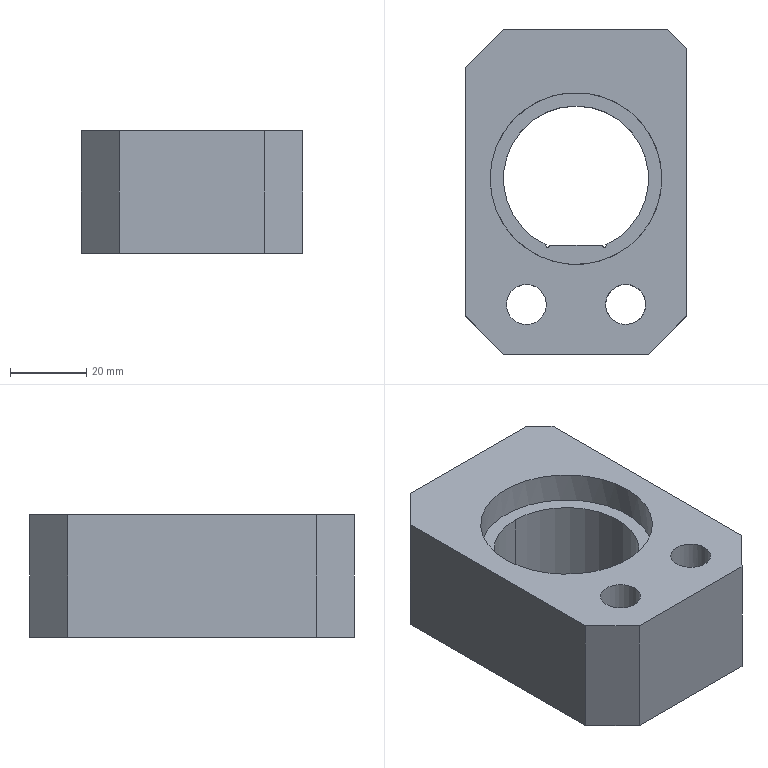Part | STEP file | lll_id3674_x_t | 1 solid | 23 faces | box 58 x 85 x 32 mm | volume 102639 mm3 | plane 14 | cylinder 9 | commonest cylinder face diameters 1 x2 10.5 x2 17 x2 38 x2 45 x1
STEP:
#1=CARTESIAN_POINT('',(3397.,-57.,84.5));
#2=VERTEX_POINT('',#1);
#3=CARTESIAN_POINT('',(3419.5,-57.,84.5));
#4=DIRECTION('',(0.,0.,-1.));
#5=DIRECTION('',(-1.,0.,0.));
#6=AXIS2_PLACEMENT_3D('',#3,#4,#5);
#7=CIRCLE('',#6,22.5);
#8=EDGE_CURVE('',#2,#2,#7,.T.);
#9=ORIENTED_EDGE('',*,*,#8,.F.);
#10=EDGE_LOOP('',(#9));
#11=FACE_BOUND('',#10,.T.);
#12=CARTESIAN_POINT('',(3426.399,-74.5,84.5));
#13=VERTEX_POINT('',#12);
#14=CARTESIAN_POINT('',(3427.357,-74.299,84.5));
#15=VERTEX_POINT('',#14);
#16=CARTESIAN_POINT('',(3426.899,-74.5,84.5));
#17=DIRECTION('',(0.,0.,1.));
#18=DIRECTION('',(-1.,0.,0.));
#19=AXIS2_PLACEMENT_3D('',#16,#17,#18);
#20=CIRCLE('',#19,0.5);
#21=EDGE_CURVE('',#13,#15,#20,.T.);
#22=ORIENTED_EDGE('',*,*,#21,.F.);
#23=CARTESIAN_POINT('',(3412.601,-74.5,84.5));
#24=VERTEX_POINT('',#23);
#25=CARTESIAN_POINT('',(3399.25,-74.5,84.5));
#26=DIRECTION('',(-1.,0.,0.));
#27=VECTOR('',#26,1.);
#28=LINE('',#25,#27);
#29=EDGE_CURVE('',#13,#24,#28,.T.);
#30=ORIENTED_EDGE('',*,*,#29,.T.);
#31=CARTESIAN_POINT('',(3411.643,-74.299,84.5));
#32=VERTEX_POINT('',#31);
#33=CARTESIAN_POINT('',(3412.101,-74.5,84.5));
#34=DIRECTION('',(0.,0.,-1.));
#35=DIRECTION('',(1.,0.,0.));
#36=AXIS2_PLACEMENT_3D('',#33,#34,#35);
#37=CIRCLE('',#36,0.5);
#38=EDGE_CURVE('',#24,#32,#37,.T.);
#39=ORIENTED_EDGE('',*,*,#38,.T.);
#40=CARTESIAN_POINT('',(3419.5,-38.,84.5));
#41=VERTEX_POINT('',#40);
#42=CARTESIAN_POINT('',(3419.5,-57.,84.5));
#43=DIRECTION('',(0.,0.,1.));
#44=DIRECTION('',(0.,1.,0.));
#45=AXIS2_PLACEMENT_3D('',#42,#43,#44);
#46=CIRCLE('',#45,19.);
#47=EDGE_CURVE('',#41,#32,#46,.T.);
#48=ORIENTED_EDGE('',*,*,#47,.F.);
#49=CARTESIAN_POINT('',(3419.5,-57.,84.5));
#50=DIRECTION('',(0.,0.,1.));
#51=DIRECTION('',(0.,1.,0.));
#52=AXIS2_PLACEMENT_3D('',#49,#50,#51);
#53=CIRCLE('',#52,19.);
#54=EDGE_CURVE('',#15,#41,#53,.T.);
#55=ORIENTED_EDGE('',*,*,#54,.F.);
#56=EDGE_LOOP('',(#22,#30,#39,#48,#55));
#57=FACE_BOUND('',#56,.T.);
#58=CARTESIAN_POINT('',(3399.25,-57.,84.5));
#59=DIRECTION('',(0.,0.,-1.));
#60=DIRECTION('',(-1.,0.,0.));
#61=AXIS2_PLACEMENT_3D('',#58,#59,#60);
#62=PLANE('',#61);
#63=ADVANCED_FACE('',(#11,#57),#62,.F.);
#64=CARTESIAN_POINT('',(3406.5,-84.75,77.5));
#65=VERTEX_POINT('',#64);
#66=CARTESIAN_POINT('',(3406.5,-90.,77.5));
#67=DIRECTION('',(0.,0.,1.));
#68=DIRECTION('',(0.,1.,0.));
#69=AXIS2_PLACEMENT_3D('',#66,#67,#68);
#70=CIRCLE('',#69,5.25);
#71=EDGE_CURVE('',#65,#65,#70,.T.);
#72=ORIENTED_EDGE('',*,*,#71,.T.);
#73=EDGE_LOOP('',(#72));
#74=FACE_BOUND('',#73,.T.);
#75=CARTESIAN_POINT('',(3406.5,-81.5,77.5));
#76=VERTEX_POINT('',#75);
#77=CARTESIAN_POINT('',(3406.5,-90.,77.5));
#78=DIRECTION('',(0.,0.,1.));
#79=DIRECTION('',(0.,1.,0.));
#80=AXIS2_PLACEMENT_3D('',#77,#78,#79);
#81=CIRCLE('',#80,8.5);
#82=EDGE_CURVE('',#76,#76,#81,.T.);
#83=ORIENTED_EDGE('',*,*,#82,.F.);
#84=EDGE_LOOP('',(#83));
#85=FACE_BOUND('',#84,.T.);
#86=CARTESIAN_POINT('',(3406.5,-90.,77.5));
#87=DIRECTION('',(0.,0.,1.));
#88=DIRECTION('',(1.,0.,0.));
#89=AXIS2_PLACEMENT_3D('',#86,#87,#88);
#90=PLANE('',#89);
#91=ADVANCED_FACE('',(#74,#85),#90,.F.);
#92=ORIENTED_EDGE('',*,*,#82,.T.);
#93=EDGE_LOOP('',(#92));
#94=FACE_BOUND('',#93,.T.);
#95=CARTESIAN_POINT('',(3406.5,-81.5,60.5));
#96=VERTEX_POINT('',#95);
#97=CARTESIAN_POINT('',(3406.5,-90.,60.5));
#98=DIRECTION('',(0.,0.,-1.));
#99=DIRECTION('',(0.,1.,0.));
#100=AXIS2_PLACEMENT_3D('',#97,#98,#99);
#101=CIRCLE('',#100,8.5);
#102=EDGE_CURVE('',#96,#96,#101,.T.);
#103=ORIENTED_EDGE('',*,*,#102,.T.);
#104=EDGE_LOOP('',(#103));
#105=FACE_BOUND('',#104,.T.);
#106=CARTESIAN_POINT('',(3406.5,-90.,60.5));
#107=DIRECTION('',(0.,0.,1.));
#108=DIRECTION('',(1.,0.,0.));
#109=AXIS2_PLACEMENT_3D('',#106,#107,#108);
#110=CYLINDRICAL_SURFACE('',#109,8.5);
#111=ADVANCED_FACE('',(#94,#105),#110,.F.);
#112=CARTESIAN_POINT('',(3400.5,-103.,60.5));
#113=VERTEX_POINT('',#112);
#114=CARTESIAN_POINT('',(3390.5,-93.,60.5));
#115=VERTEX_POINT('',#114);
#116=CARTESIAN_POINT('',(3430.983,-133.483,60.5));
#117=DIRECTION('',(-0.7071,0.7071,0.));
#118=VECTOR('',#117,1.);
#119=LINE('',#116,#118);
#120=EDGE_CURVE('',#113,#115,#119,.T.);
#121=ORIENTED_EDGE('',*,*,#120,.F.);
#122=CARTESIAN_POINT('',(3400.5,-103.,92.5));
#123=VERTEX_POINT('',#122);
#124=CARTESIAN_POINT('',(3400.5,-103.,-8.5));
#125=DIRECTION('',(0.,0.,-1.));
#126=VECTOR('',#125,1.);
#127=LINE('',#124,#126);
#128=EDGE_CURVE('',#123,#113,#127,.T.);
#129=ORIENTED_EDGE('',*,*,#128,.F.);
#130=CARTESIAN_POINT('',(3390.5,-93.,92.5));
#131=VERTEX_POINT('',#130);
#132=CARTESIAN_POINT('',(3435.933,-138.433,92.5));
#133=DIRECTION('',(0.7071,-0.7071,0.));
#134=VECTOR('',#133,1.);
#135=LINE('',#132,#134);
#136=EDGE_CURVE('',#131,#123,#135,.T.);
#137=ORIENTED_EDGE('',*,*,#136,.F.);
#138=CARTESIAN_POINT('',(3390.5,-93.,-8.5));
#139=DIRECTION('',(0.,0.,1.));
#140=VECTOR('',#139,1.);
#141=LINE('',#138,#140);
#142=EDGE_CURVE('',#115,#131,#141,.T.);
#143=ORIENTED_EDGE('',*,*,#142,.F.);
#144=EDGE_LOOP('',(#121,#129,#137,#143));
#145=FACE_OUTER_BOUND('',#144,.T.);
#146=CARTESIAN_POINT('',(3390.5,-93.,-8.5));
#147=DIRECTION('',(0.7071,0.7071,0.));
#148=DIRECTION('',(0.,0.,1.));
#149=AXIS2_PLACEMENT_3D('',#146,#147,#148);
#150=PLANE('',#149);
#151=ADVANCED_FACE('',(#145),#150,.F.);
#152=CARTESIAN_POINT('',(3390.5,-28.,60.5));
#153=VERTEX_POINT('',#152);
#154=CARTESIAN_POINT('',(3390.5,-83.276,60.5));
#155=DIRECTION('',(0.,1.,0.));
#156=VECTOR('',#155,1.);
#157=LINE('',#154,#156);
#158=EDGE_CURVE('',#115,#153,#157,.T.);
#159=ORIENTED_EDGE('',*,*,#158,.F.);
#160=ORIENTED_EDGE('',*,*,#142,.T.);
#161=CARTESIAN_POINT('',(3390.5,-28.,92.5));
#162=VERTEX_POINT('',#161);
#163=CARTESIAN_POINT('',(3390.5,-88.225,92.5));
#164=DIRECTION('',(0.,-1.,0.));
#165=VECTOR('',#164,1.);
#166=LINE('',#163,#165);
#167=EDGE_CURVE('',#162,#131,#166,.T.);
#168=ORIENTED_EDGE('',*,*,#167,.F.);
#169=CARTESIAN_POINT('',(3390.5,-28.,-8.5));
#170=DIRECTION('',(0.,0.,-1.));
#171=VECTOR('',#170,1.);
#172=LINE('',#169,#171);
#173=EDGE_CURVE('',#162,#153,#172,.T.);
#174=ORIENTED_EDGE('',*,*,#173,.T.);
#175=EDGE_LOOP('',(#159,#160,#168,#174));
#176=FACE_OUTER_BOUND('',#175,.T.);
#177=CARTESIAN_POINT('',(3390.5,-52.05,-8.5));
#178=DIRECTION('',(-1.,0.,0.));
#179=DIRECTION('',(0.,0.,1.));
#180=AXIS2_PLACEMENT_3D('',#177,#178,#179);
#181=PLANE('',#180);
#182=ADVANCED_FACE('',(#176),#181,.T.);
#183=CARTESIAN_POINT('',(3400.5,-18.,92.5));
#184=VERTEX_POINT('',#183);
#185=CARTESIAN_POINT('',(3414.207,-4.293,92.5));
#186=DIRECTION('',(-0.7071,-0.7071,0.));
#187=VECTOR('',#186,1.);
#188=LINE('',#185,#187);
#189=EDGE_CURVE('',#184,#162,#188,.T.);
#190=ORIENTED_EDGE('',*,*,#189,.F.);
#191=CARTESIAN_POINT('',(3400.5,-18.,60.5));
#192=VERTEX_POINT('',#191);
#193=CARTESIAN_POINT('',(3400.5,-18.,-8.5));
#194=DIRECTION('',(0.,0.,1.));
#195=VECTOR('',#194,1.);
#196=LINE('',#193,#195);
#197=EDGE_CURVE('',#192,#184,#196,.T.);
#198=ORIENTED_EDGE('',*,*,#197,.F.);
#199=CARTESIAN_POINT('',(3414.207,-4.293,60.5));
#200=DIRECTION('',(0.7071,0.7071,0.));
#201=VECTOR('',#200,1.);
#202=LINE('',#199,#201);
#203=EDGE_CURVE('',#153,#192,#202,.T.);
#204=ORIENTED_EDGE('',*,*,#203,.F.);
#205=ORIENTED_EDGE('',*,*,#173,.F.);
#206=EDGE_LOOP('',(#190,#198,#204,#205));
#207=FACE_OUTER_BOUND('',#206,.T.);
#208=CARTESIAN_POINT('',(3390.5,-28.,-8.5));
#209=DIRECTION('',(0.7071,-0.7071,0.));
#210=DIRECTION('',(0.,0.,-1.));
#211=AXIS2_PLACEMENT_3D('',#208,#209,#210);
#212=PLANE('',#211);
#213=ADVANCED_FACE('',(#207),#212,.F.);
#214=CARTESIAN_POINT('',(3443.5,-18.,92.5));
#215=VERTEX_POINT('',#214);
#216=CARTESIAN_POINT('',(3487.64,-18.,92.5));
#217=DIRECTION('',(-1.,0.,0.));
#218=VECTOR('',#217,1.);
#219=LINE('',#216,#218);
#220=EDGE_CURVE('',#215,#184,#219,.T.);
#221=ORIENTED_EDGE('',*,*,#220,.F.);
#222=CARTESIAN_POINT('',(3443.5,-18.,60.5));
#223=VERTEX_POINT('',#222);
#224=CARTESIAN_POINT('',(3443.5,-18.,-8.5));
#225=DIRECTION('',(0.,0.,-1.));
#226=VECTOR('',#225,1.);
#227=LINE('',#224,#226);
#228=EDGE_CURVE('',#215,#223,#227,.T.);
#229=ORIENTED_EDGE('',*,*,#228,.T.);
#230=CARTESIAN_POINT('',(3482.69,-18.,60.5));
#231=DIRECTION('',(1.,0.,0.));
#232=VECTOR('',#231,1.);
#233=LINE('',#230,#232);
#234=EDGE_CURVE('',#192,#223,#233,.T.);
#235=ORIENTED_EDGE('',*,*,#234,.F.);
#236=ORIENTED_EDGE('',*,*,#197,.T.);
#237=EDGE_LOOP('',(#221,#229,#235,#236));
#238=FACE_OUTER_BOUND('',#237,.T.);
#239=CARTESIAN_POINT('',(3419.5,-18.,-8.5));
#240=DIRECTION('',(0.,1.,0.));
#241=DIRECTION('',(0.,0.,-1.));
#242=AXIS2_PLACEMENT_3D('',#239,#240,#241);
#243=PLANE('',#242);
#244=ADVANCED_FACE('',(#238),#243,.T.);
#245=CARTESIAN_POINT('',(3448.5,-23.,92.5));
#246=VERTEX_POINT('',#245);
#247=CARTESIAN_POINT('',(3495.433,-69.933,92.5));
#248=DIRECTION('',(-0.7071,0.7071,0.));
#249=VECTOR('',#248,1.);
#250=LINE('',#247,#249);
#251=EDGE_CURVE('',#246,#215,#250,.T.);
#252=ORIENTED_EDGE('',*,*,#251,.F.);
#253=CARTESIAN_POINT('',(3448.5,-23.,60.5));
#254=VERTEX_POINT('',#253);
#255=CARTESIAN_POINT('',(3448.5,-23.,-8.5));
#256=DIRECTION('',(0.,0.,1.));
#257=VECTOR('',#256,1.);
#258=LINE('',#255,#257);
#259=EDGE_CURVE('',#254,#246,#258,.T.);
#260=ORIENTED_EDGE('',*,*,#259,.F.);
#261=CARTESIAN_POINT('',(3490.483,-64.983,60.5));
#262=DIRECTION('',(0.7071,-0.7071,0.));
#263=VECTOR('',#262,1.);
#264=LINE('',#261,#263);
#265=EDGE_CURVE('',#223,#254,#264,.T.);
#266=ORIENTED_EDGE('',*,*,#265,.F.);
#267=ORIENTED_EDGE('',*,*,#228,.F.);
#268=EDGE_LOOP('',(#252,#260,#266,#267));
#269=FACE_OUTER_BOUND('',#268,.T.);
#270=CARTESIAN_POINT('',(3443.5,-18.,-8.5));
#271=DIRECTION('',(-0.7071,-0.7071,0.));
#272=DIRECTION('',(0.,0.,-1.));
#273=AXIS2_PLACEMENT_3D('',#270,#271,#272);
#274=PLANE('',#273);
#275=ADVANCED_FACE('',(#269),#274,.F.);
#276=CARTESIAN_POINT('',(3448.5,-93.,92.5));
#277=VERTEX_POINT('',#276);
#278=CARTESIAN_POINT('',(3448.5,-88.225,92.5));
#279=DIRECTION('',(0.,1.,0.));
#280=VECTOR('',#279,1.);
#281=LINE('',#278,#280);
#282=EDGE_CURVE('',#277,#246,#281,.T.);
#283=ORIENTED_EDGE('',*,*,#282,.F.);
#284=CARTESIAN_POINT('',(3448.5,-93.,60.5));
#285=VERTEX_POINT('',#284);
#286=CARTESIAN_POINT('',(3448.5,-93.,-8.5));
#287=DIRECTION('',(0.,0.,-1.));
#288=VECTOR('',#287,1.);
#289=LINE('',#286,#288);
#290=EDGE_CURVE('',#277,#285,#289,.T.);
#291=ORIENTED_EDGE('',*,*,#290,.T.);
#292=CARTESIAN_POINT('',(3448.5,-83.276,60.5));
#293=DIRECTION('',(0.,-1.,0.));
#294=VECTOR('',#293,1.);
#295=LINE('',#292,#294);
#296=EDGE_CURVE('',#254,#285,#295,.T.);
#297=ORIENTED_EDGE('',*,*,#296,.F.);
#298=ORIENTED_EDGE('',*,*,#259,.T.);
#299=EDGE_LOOP('',(#283,#291,#297,#298));
#300=FACE_OUTER_BOUND('',#299,.T.);
#301=CARTESIAN_POINT('',(3448.5,-57.,-8.5));
#302=DIRECTION('',(1.,0.,0.));
#303=DIRECTION('',(0.,0.,-1.));
#304=AXIS2_PLACEMENT_3D('',#301,#302,#303);
#305=PLANE('',#304);
#306=ADVANCED_FACE('',(#300),#305,.T.);
#307=CARTESIAN_POINT('',(3438.5,-103.,92.5));
#308=VERTEX_POINT('',#307);
#309=CARTESIAN_POINT('',(3470.707,-70.793,92.5));
#310=DIRECTION('',(0.7071,0.7071,0.));
#311=VECTOR('',#310,1.);
#312=LINE('',#309,#311);
#313=EDGE_CURVE('',#308,#277,#312,.T.);
#314=ORIENTED_EDGE('',*,*,#313,.F.);
#315=CARTESIAN_POINT('',(3438.5,-103.,60.5));
#316=VERTEX_POINT('',#315);
#317=CARTESIAN_POINT('',(3438.5,-103.,-8.5));
#318=DIRECTION('',(0.,0.,1.));
#319=VECTOR('',#318,1.);
#320=LINE('',#317,#319);
#321=EDGE_CURVE('',#316,#308,#320,.T.);
#322=ORIENTED_EDGE('',*,*,#321,.F.);
#323=CARTESIAN_POINT('',(3470.707,-70.793,60.5));
#324=DIRECTION('',(-0.7071,-0.7071,0.));
#325=VECTOR('',#324,1.);
#326=LINE('',#323,#325);
#327=EDGE_CURVE('',#285,#316,#326,.T.);
#328=ORIENTED_EDGE('',*,*,#327,.F.);
#329=ORIENTED_EDGE('',*,*,#290,.F.);
#330=EDGE_LOOP('',(#314,#322,#328,#329));
#331=FACE_OUTER_BOUND('',#330,.T.);
#332=CARTESIAN_POINT('',(3448.5,-93.,-8.5));
#333=DIRECTION('',(-0.7071,0.7071,0.));
#334=DIRECTION('',(0.,0.,-1.));
#335=AXIS2_PLACEMENT_3D('',#332,#333,#334);
#336=PLANE('',#335);
#337=ADVANCED_FACE('',(#331),#336,.F.);
#338=CARTESIAN_POINT('',(3482.69,-103.,60.5));
#339=DIRECTION('',(-1.,0.,0.));
#340=VECTOR('',#339,1.);
#341=LINE('',#338,#340);
#342=EDGE_CURVE('',#316,#113,#341,.T.);
#343=ORIENTED_EDGE('',*,*,#342,.F.);
#344=ORIENTED_EDGE('',*,*,#321,.T.);
#345=CARTESIAN_POINT('',(3487.64,-103.,92.5));
#346=DIRECTION('',(1.,0.,0.));
#347=VECTOR('',#346,1.);
#348=LINE('',#345,#347);
#349=EDGE_CURVE('',#123,#308,#348,.T.);
#350=ORIENTED_EDGE('',*,*,#349,.F.);
#351=ORIENTED_EDGE('',*,*,#128,.T.);
#352=EDGE_LOOP('',(#343,#344,#350,#351));
#353=FACE_OUTER_BOUND('',#352,.T.);
#354=CARTESIAN_POINT('',(3419.5,-103.,-8.5));
#355=DIRECTION('',(0.,-1.,0.));
#356=DIRECTION('',(0.,0.,1.));
#357=AXIS2_PLACEMENT_3D('',#354,#355,#356);
#358=PLANE('',#357);
#359=ADVANCED_FACE('',(#353),#358,.T.);
#360=CARTESIAN_POINT('',(3406.5,-84.75,92.5));
#361=VERTEX_POINT('',#360);
#362=CARTESIAN_POINT('',(3406.5,-90.,92.5));
#363=DIRECTION('',(0.,0.,-1.));
#364=DIRECTION('',(0.,1.,0.));
#365=AXIS2_PLACEMENT_3D('',#362,#363,#364);
#366=CIRCLE('',#365,5.25);
#367=EDGE_CURVE('',#361,#361,#366,.T.);
#368=ORIENTED_EDGE('',*,*,#367,.F.);
#369=EDGE_LOOP('',(#368));
#370=FACE_BOUND('',#369,.T.);
#371=ORIENTED_EDGE('',*,*,#71,.F.);
#372=EDGE_LOOP('',(#371));
#373=FACE_BOUND('',#372,.T.);
#374=CARTESIAN_POINT('',(3406.5,-90.,160.5));
#375=DIRECTION('',(0.,0.,1.));
#376=DIRECTION('',(1.,0.,0.));
#377=AXIS2_PLACEMENT_3D('',#374,#375,#376);
#378=CYLINDRICAL_SURFACE('',#377,5.25);
#379=ADVANCED_FACE('',(#370,#373),#378,.F.);
#380=ORIENTED_EDGE('',*,*,#8,.T.);
#381=EDGE_LOOP('',(#380));
#382=FACE_BOUND('',#381,.T.);
#383=CARTESIAN_POINT('',(3442.,-57.,92.5));
#384=VERTEX_POINT('',#383);
#385=CARTESIAN_POINT('',(3419.5,-57.,92.5));
#386=DIRECTION('',(0.,0.,1.));
#387=DIRECTION('',(1.,0.,0.));
#388=AXIS2_PLACEMENT_3D('',#385,#386,#387);
#389=CIRCLE('',#388,22.5);
#390=EDGE_CURVE('',#384,#384,#389,.T.);
#391=ORIENTED_EDGE('',*,*,#390,.T.);
#392=EDGE_LOOP('',(#391));
#393=FACE_BOUND('',#392,.T.);
#394=CARTESIAN_POINT('',(3419.5,-57.,88.5));
#395=DIRECTION('',(0.,0.,-1.));
#396=DIRECTION('',(0.,-1.,0.));
#397=AXIS2_PLACEMENT_3D('',#394,#395,#396);
#398=CYLINDRICAL_SURFACE('',#397,22.5);
#399=ADVANCED_FACE('',(#382,#393),#398,.F.);
#400=CARTESIAN_POINT('',(3437.75,-90.,92.5));
#401=VERTEX_POINT('',#400);
#402=CARTESIAN_POINT('',(3432.5,-90.,92.5));
#403=DIRECTION('',(0.,0.,1.));
#404=DIRECTION('',(1.,0.,0.));
#405=AXIS2_PLACEMENT_3D('',#402,#403,#404);
#406=CIRCLE('',#405,5.25);
#407=EDGE_CURVE('',#401,#401,#406,.T.);
#408=ORIENTED_EDGE('',*,*,#407,.F.);
#409=EDGE_LOOP('',(#408));
#410=FACE_BOUND('',#409,.T.);
#411=ORIENTED_EDGE('',*,*,#390,.F.);
#412=EDGE_LOOP('',(#411));
#413=FACE_BOUND('',#412,.T.);
#414=ORIENTED_EDGE('',*,*,#367,.T.);
#415=EDGE_LOOP('',(#414));
#416=FACE_BOUND('',#415,.T.);
#417=ORIENTED_EDGE('',*,*,#349,.T.);
#418=ORIENTED_EDGE('',*,*,#313,.T.);
#419=ORIENTED_EDGE('',*,*,#282,.T.);
#420=ORIENTED_EDGE('',*,*,#251,.T.);
#421=ORIENTED_EDGE('',*,*,#220,.T.);
#422=ORIENTED_EDGE('',*,*,#189,.T.);
#423=ORIENTED_EDGE('',*,*,#167,.T.);
#424=ORIENTED_EDGE('',*,*,#136,.T.);
#425=EDGE_LOOP('',(#417,#418,#419,#420,#421,#422,#423,#424));
#426=FACE_BOUND('',#425,.T.);
#427=CARTESIAN_POINT('',(3487.64,-88.225,92.5));
#428=DIRECTION('',(0.,0.,1.));
#429=DIRECTION('',(1.,0.,0.));
#430=AXIS2_PLACEMENT_3D('',#427,#428,#429);
#431=PLANE('',#430);
#432=ADVANCED_FACE('',(#410,#413,#416,#426),#431,.T.);
#433=CARTESIAN_POINT('',(3427.357,-74.299,60.5));
#434=VERTEX_POINT('',#433);
#435=CARTESIAN_POINT('',(3426.399,-74.5,60.5));
#436=VERTEX_POINT('',#435);
#437=CARTESIAN_POINT('',(3426.899,-74.5,60.5));
#438=DIRECTION('',(0.,0.,-1.));
#439=DIRECTION('',(1.,0.,0.));
#440=AXIS2_PLACEMENT_3D('',#437,#438,#439);
#441=CIRCLE('',#440,0.5);
#442=EDGE_CURVE('',#434,#436,#441,.T.);
#443=ORIENTED_EDGE('',*,*,#442,.F.);
#444=CARTESIAN_POINT('',(3419.5,-38.,60.5));
#445=VERTEX_POINT('',#444);
#446=CARTESIAN_POINT('',(3419.5,-57.,60.5));
#447=DIRECTION('',(0.,0.,-1.));
#448=DIRECTION('',(1.,0.,0.));
#449=AXIS2_PLACEMENT_3D('',#446,#447,#448);
#450=CIRCLE('',#449,19.);
#451=EDGE_CURVE('',#445,#434,#450,.T.);
#452=ORIENTED_EDGE('',*,*,#451,.F.);
#453=CARTESIAN_POINT('',(3411.643,-74.299,60.5));
#454=VERTEX_POINT('',#453);
#455=CARTESIAN_POINT('',(3419.5,-57.,60.5));
#456=DIRECTION('',(0.,0.,-1.));
#457=DIRECTION('',(1.,0.,0.));
#458=AXIS2_PLACEMENT_3D('',#455,#456,#457);
#459=CIRCLE('',#458,19.);
#460=EDGE_CURVE('',#454,#445,#459,.T.);
#461=ORIENTED_EDGE('',*,*,#460,.F.);
#462=CARTESIAN_POINT('',(3412.601,-74.5,60.5));
#463=VERTEX_POINT('',#462);
#464=CARTESIAN_POINT('',(3412.101,-74.5,60.5));
#465=DIRECTION('',(0.,0.,-1.));
#466=DIRECTION('',(1.,0.,0.));
#467=AXIS2_PLACEMENT_3D('',#464,#465,#466);
#468=CIRCLE('',#467,0.5);
#469=EDGE_CURVE('',#463,#454,#468,.T.);
#470=ORIENTED_EDGE('',*,*,#469,.F.);
#471=CARTESIAN_POINT('',(3482.69,-74.5,60.5));
#472=DIRECTION('',(-1.,0.,0.));
#473=VECTOR('',#472,1.);
#474=LINE('',#471,#473);
#475=EDGE_CURVE('',#436,#463,#474,.T.);
#476=ORIENTED_EDGE('',*,*,#475,.F.);
#477=EDGE_LOOP('',(#443,#452,#461,#470,#476));
#478=FACE_BOUND('',#477,.T.);
#479=CARTESIAN_POINT('',(3441.,-90.,60.5));
#480=VERTEX_POINT('',#479);
#481=CARTESIAN_POINT('',(3432.5,-90.,60.5));
#482=DIRECTION('',(0.,0.,-1.));
#483=DIRECTION('',(1.,0.,0.));
#484=AXIS2_PLACEMENT_3D('',#481,#482,#483);
#485=CIRCLE('',#484,8.5);
#486=EDGE_CURVE('',#480,#480,#485,.T.);
#487=ORIENTED_EDGE('',*,*,#486,.F.);
#488=EDGE_LOOP('',(#487));
#489=FACE_BOUND('',#488,.T.);
#490=ORIENTED_EDGE('',*,*,#296,.T.);
#491=ORIENTED_EDGE('',*,*,#327,.T.);
#492=ORIENTED_EDGE('',*,*,#342,.T.);
#493=ORIENTED_EDGE('',*,*,#120,.T.);
#494=ORIENTED_EDGE('',*,*,#158,.T.);
#495=ORIENTED_EDGE('',*,*,#203,.T.);
#496=ORIENTED_EDGE('',*,*,#234,.T.);
#497=ORIENTED_EDGE('',*,*,#265,.T.);
#498=EDGE_LOOP('',(#490,#491,#492,#493,#494,#495,#496,#497));
#499=FACE_BOUND('',#498,.T.);
#500=ORIENTED_EDGE('',*,*,#102,.F.);
#501=EDGE_LOOP('',(#500));
#502=FACE_BOUND('',#501,.T.);
#503=CARTESIAN_POINT('',(3482.69,-83.276,60.5));
#504=DIRECTION('',(0.,0.,1.));
#505=DIRECTION('',(1.,0.,0.));
#506=AXIS2_PLACEMENT_3D('',#503,#504,#505);
#507=PLANE('',#506);
#508=ADVANCED_FACE('',(#478,#489,#499,#502),#507,.F.);
#509=CARTESIAN_POINT('',(3432.5,-84.75,77.5));
#510=VERTEX_POINT('',#509);
#511=CARTESIAN_POINT('',(3432.5,-90.,77.5));
#512=DIRECTION('',(0.,0.,1.));
#513=DIRECTION('',(0.,1.,0.));
#514=AXIS2_PLACEMENT_3D('',#511,#512,#513);
#515=CIRCLE('',#514,5.25);
#516=EDGE_CURVE('',#510,#510,#515,.T.);
#517=ORIENTED_EDGE('',*,*,#516,.T.);
#518=EDGE_LOOP('',(#517));
#519=FACE_BOUND('',#518,.T.);
#520=CARTESIAN_POINT('',(3432.5,-81.5,77.5));
#521=VERTEX_POINT('',#520);
#522=CARTESIAN_POINT('',(3432.5,-90.,77.5));
#523=DIRECTION('',(0.,0.,1.));
#524=DIRECTION('',(0.,1.,0.));
#525=AXIS2_PLACEMENT_3D('',#522,#523,#524);
#526=CIRCLE('',#525,8.5);
#527=EDGE_CURVE('',#521,#521,#526,.T.);
#528=ORIENTED_EDGE('',*,*,#527,.F.);
#529=EDGE_LOOP('',(#528));
#530=FACE_BOUND('',#529,.T.);
#531=CARTESIAN_POINT('',(3432.5,-90.,77.5));
#532=DIRECTION('',(0.,0.,1.));
#533=DIRECTION('',(-1.,0.,0.));
#534=AXIS2_PLACEMENT_3D('',#531,#532,#533);
#535=PLANE('',#534);
#536=ADVANCED_FACE('',(#519,#530),#535,.F.);
#537=ORIENTED_EDGE('',*,*,#407,.T.);
#538=EDGE_LOOP('',(#537));
#539=FACE_BOUND('',#538,.T.);
#540=ORIENTED_EDGE('',*,*,#516,.F.);
#541=EDGE_LOOP('',(#540));
#542=FACE_BOUND('',#541,.T.);
#543=CARTESIAN_POINT('',(3432.5,-90.,160.5));
#544=DIRECTION('',(0.,0.,1.));
#545=DIRECTION('',(-1.,0.,0.));
#546=AXIS2_PLACEMENT_3D('',#543,#544,#545);
#547=CYLINDRICAL_SURFACE('',#546,5.25);
#548=ADVANCED_FACE('',(#539,#542),#547,.F.);
#549=ORIENTED_EDGE('',*,*,#527,.T.);
#550=EDGE_LOOP('',(#549));
#551=FACE_BOUND('',#550,.T.);
#552=ORIENTED_EDGE('',*,*,#486,.T.);
#553=EDGE_LOOP('',(#552));
#554=FACE_BOUND('',#553,.T.);
#555=CARTESIAN_POINT('',(3432.5,-90.,60.5));
#556=DIRECTION('',(0.,0.,1.));
#557=DIRECTION('',(-1.,0.,0.));
#558=AXIS2_PLACEMENT_3D('',#555,#556,#557);
#559=CYLINDRICAL_SURFACE('',#558,8.5);
#560=ADVANCED_FACE('',(#551,#554),#559,.F.);
#561=ORIENTED_EDGE('',*,*,#29,.F.);
#562=CARTESIAN_POINT('',(3426.399,-74.5,84.5));
#563=DIRECTION('',(0.,0.,-1.));
#564=VECTOR('',#563,1.);
#565=LINE('',#562,#564);
#566=EDGE_CURVE('',#13,#436,#565,.T.);
#567=ORIENTED_EDGE('',*,*,#566,.T.);
#568=ORIENTED_EDGE('',*,*,#475,.T.);
#569=CARTESIAN_POINT('',(3412.601,-74.5,84.5));
#570=DIRECTION('',(0.,0.,1.));
#571=VECTOR('',#570,1.);
#572=LINE('',#569,#571);
#573=EDGE_CURVE('',#463,#24,#572,.T.);
#574=ORIENTED_EDGE('',*,*,#573,.T.);
#575=EDGE_LOOP('',(#561,#567,#568,#574));
#576=FACE_OUTER_BOUND('',#575,.T.);
#577=CARTESIAN_POINT('',(3419.5,-74.5,88.5));
#578=DIRECTION('',(0.,-1.,0.));
#579=DIRECTION('',(0.,0.,-1.));
#580=AXIS2_PLACEMENT_3D('',#577,#578,#579);
#581=PLANE('',#580);
#582=ADVANCED_FACE('',(#576),#581,.F.);
#583=ORIENTED_EDGE('',*,*,#47,.T.);
#584=CARTESIAN_POINT('',(3411.643,-74.299,67.));
#585=DIRECTION('',(0.,0.,-1.));
#586=VECTOR('',#585,1.);
#587=LINE('',#584,#586);
#588=EDGE_CURVE('',#32,#454,#587,.T.);
#589=ORIENTED_EDGE('',*,*,#588,.T.);
#590=ORIENTED_EDGE('',*,*,#460,.T.);
#591=CARTESIAN_POINT('',(3419.5,-38.,38.5));
#592=DIRECTION('',(0.,0.,-1.));
#593=VECTOR('',#592,1.);
#594=LINE('',#591,#593);
#595=EDGE_CURVE('',#41,#445,#594,.T.);
#596=ORIENTED_EDGE('',*,*,#595,.F.);
#597=EDGE_LOOP('',(#583,#589,#590,#596));
#598=FACE_OUTER_BOUND('',#597,.T.);
#599=CARTESIAN_POINT('',(3419.5,-57.,38.5));
#600=DIRECTION('',(0.,0.,-1.));
#601=DIRECTION('',(0.,-1.,0.));
#602=AXIS2_PLACEMENT_3D('',#599,#600,#601);
#603=CYLINDRICAL_SURFACE('',#602,19.);
#604=ADVANCED_FACE('',(#598),#603,.F.);
#605=ORIENTED_EDGE('',*,*,#451,.T.);
#606=CARTESIAN_POINT('',(3427.357,-74.299,67.));
#607=DIRECTION('',(0.,0.,1.));
#608=VECTOR('',#607,1.);
#609=LINE('',#606,#608);
#610=EDGE_CURVE('',#434,#15,#609,.T.);
#611=ORIENTED_EDGE('',*,*,#610,.T.);
#612=ORIENTED_EDGE('',*,*,#54,.T.);
#613=ORIENTED_EDGE('',*,*,#595,.T.);
#614=EDGE_LOOP('',(#605,#611,#612,#613));
#615=FACE_OUTER_BOUND('',#614,.T.);
#616=CARTESIAN_POINT('',(3419.5,-57.,38.5));
#617=DIRECTION('',(0.,0.,-1.));
#618=DIRECTION('',(0.,-1.,0.));
#619=AXIS2_PLACEMENT_3D('',#616,#617,#618);
#620=CYLINDRICAL_SURFACE('',#619,19.);
#621=ADVANCED_FACE('',(#615),#620,.F.);
#622=ORIENTED_EDGE('',*,*,#469,.T.);
#623=ORIENTED_EDGE('',*,*,#588,.F.);
#624=ORIENTED_EDGE('',*,*,#38,.F.);
#625=ORIENTED_EDGE('',*,*,#573,.F.);
#626=EDGE_LOOP('',(#622,#623,#624,#625));
#627=FACE_OUTER_BOUND('',#626,.T.);
#628=CARTESIAN_POINT('',(3412.101,-74.5,84.5));
#629=DIRECTION('',(0.,0.,-1.));
#630=DIRECTION('',(1.,0.,0.));
#631=AXIS2_PLACEMENT_3D('',#628,#629,#630);
#632=CYLINDRICAL_SURFACE('',#631,0.5);
#633=ADVANCED_FACE('',(#627),#632,.F.);
#634=ORIENTED_EDGE('',*,*,#21,.T.);
#635=ORIENTED_EDGE('',*,*,#610,.F.);
#636=ORIENTED_EDGE('',*,*,#442,.T.);
#637=ORIENTED_EDGE('',*,*,#566,.F.);
#638=EDGE_LOOP('',(#634,#635,#636,#637));
#639=FACE_OUTER_BOUND('',#638,.T.);
#640=CARTESIAN_POINT('',(3426.899,-74.5,84.5));
#641=DIRECTION('',(0.,0.,-1.));
#642=DIRECTION('',(-1.,0.,0.));
#643=AXIS2_PLACEMENT_3D('',#640,#641,#642);
#644=CYLINDRICAL_SURFACE('',#643,0.5);
#645=ADVANCED_FACE('',(#639),#644,.F.);
#646=CLOSED_SHELL('',(#63,#91,#111,#151,#182,#213,#244,#275,#306,#337,#359,#379,#399,#432,#508,#536,#548,#560,#582,#604,#621,#633,#645));
#647=MANIFOLD_SOLID_BREP('',#646);
#648=(LENGTH_UNIT()NAMED_UNIT(*)SI_UNIT(.MILLI.,.METRE.));
#649=UNCERTAINTY_MEASURE_WITH_UNIT(LENGTH_MEASURE(0.00002),#648,'','');
#650=(NAMED_UNIT(*)PLANE_ANGLE_UNIT()SI_UNIT($,.RADIAN.));
#651=PLANE_ANGLE_MEASURE_WITH_UNIT(PLANE_ANGLE_MEASURE(0.01745),#650);
#652=DIMENSIONAL_EXPONENTS(0.,0.,0.,0.,0.,0.,0.);
#653=(CONVERSION_BASED_UNIT('DEGREE',#651)NAMED_UNIT(#652)PLANE_ANGLE_UNIT());
#654=(NAMED_UNIT(*)SI_UNIT($,.STERADIAN.)SOLID_ANGLE_UNIT());
#655=(GEOMETRIC_REPRESENTATION_CONTEXT(3)GLOBAL_UNCERTAINTY_ASSIGNED_CONTEXT((#649))GLOBAL_UNIT_ASSIGNED_CONTEXT((#648,#653,#654))REPRESENTATION_CONTEXT('',''));
#656=ADVANCED_BREP_SHAPE_REPRESENTATION('',(#647),#655);